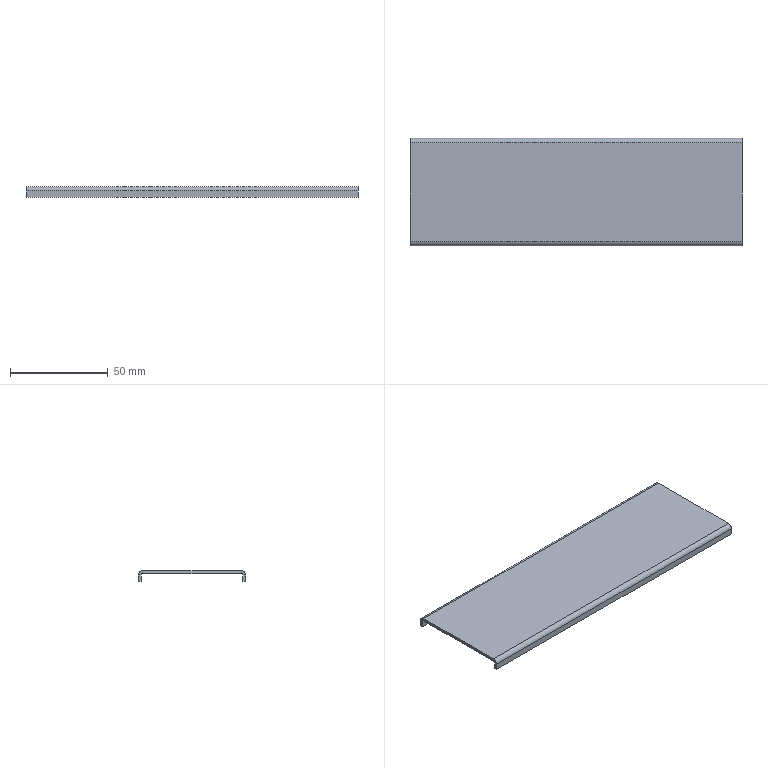Part | NX | features BREP 1 | 1 solid | 22 faces | box 170 x 55 x 5.5 mm | volume 15740 mm3 | plane 18 | cylinder 4 | commonest cylinder face diameters 1.473 x2 4.473 x2
STEP:
#1=CARTESIAN_POINT('',(85.,25.263,-1.5));
#2=VERTEX_POINT('',#1);
#3=CARTESIAN_POINT('',(-85.,25.263,-1.5));
#4=VERTEX_POINT('',#3);
#5=CARTESIAN_POINT('',(85.,25.263,-1.5));
#6=DIRECTION('',(-1.,0.,0.));
#7=VECTOR('',#6,1000.);
#8=LINE('',#5,#7);
#9=EDGE_CURVE('',#2,#4,#8,.T.);
#10=ORIENTED_EDGE('',*,*,#9,.F.);
#11=CARTESIAN_POINT('',(85.,-25.263,-1.5));
#12=VERTEX_POINT('',#11);
#13=CARTESIAN_POINT('',(85.,26.,-1.5));
#14=DIRECTION('',(0.,1.,0.));
#15=VECTOR('',#14,1000.);
#16=LINE('',#13,#15);
#17=EDGE_CURVE('',#12,#2,#16,.T.);
#18=ORIENTED_EDGE('',*,*,#17,.F.);
#19=CARTESIAN_POINT('',(-85.,-25.263,-1.5));
#20=VERTEX_POINT('',#19);
#21=CARTESIAN_POINT('',(-85.,-25.263,-1.5));
#22=DIRECTION('',(1.,0.,0.));
#23=VECTOR('',#22,1000.);
#24=LINE('',#21,#23);
#25=EDGE_CURVE('',#20,#12,#24,.T.);
#26=ORIENTED_EDGE('',*,*,#25,.F.);
#27=CARTESIAN_POINT('',(-85.,26.,-1.5));
#28=DIRECTION('',(0.,-1.,0.));
#29=VECTOR('',#28,1000.);
#30=LINE('',#27,#29);
#31=EDGE_CURVE('',#4,#20,#30,.T.);
#32=ORIENTED_EDGE('',*,*,#31,.F.);
#33=EDGE_LOOP('',(#10,#18,#26,#32));
#34=FACE_BOUND('',#33,.T.);
#35=CARTESIAN_POINT('',(0.,0.,-1.5));
#36=DIRECTION('',(0.,0.,1.));
#37=DIRECTION('',(1.,0.,0.));
#38=AXIS2_PLACEMENT_3D('',#35,#36,#37);
#39=PLANE('',#38);
#40=ADVANCED_FACE('',(#34),#39,.F.);
#41=CARTESIAN_POINT('',(85.,-25.263,0.));
#42=VERTEX_POINT('',#41);
#43=CARTESIAN_POINT('',(85.,25.263,0.));
#44=VERTEX_POINT('',#43);
#45=CARTESIAN_POINT('',(85.,26.,0.));
#46=DIRECTION('',(0.,1.,0.));
#47=VECTOR('',#46,1000.);
#48=LINE('',#45,#47);
#49=EDGE_CURVE('',#42,#44,#48,.T.);
#50=ORIENTED_EDGE('',*,*,#49,.T.);
#51=CARTESIAN_POINT('',(-85.,25.263,0.));
#52=VERTEX_POINT('',#51);
#53=CARTESIAN_POINT('',(85.,25.263,0.));
#54=DIRECTION('',(-1.,0.,0.));
#55=VECTOR('',#54,1000.);
#56=LINE('',#53,#55);
#57=EDGE_CURVE('',#44,#52,#56,.T.);
#58=ORIENTED_EDGE('',*,*,#57,.T.);
#59=CARTESIAN_POINT('',(-85.,-25.263,0.));
#60=VERTEX_POINT('',#59);
#61=CARTESIAN_POINT('',(-85.,26.,0.));
#62=DIRECTION('',(0.,-1.,0.));
#63=VECTOR('',#62,1000.);
#64=LINE('',#61,#63);
#65=EDGE_CURVE('',#52,#60,#64,.T.);
#66=ORIENTED_EDGE('',*,*,#65,.T.);
#67=CARTESIAN_POINT('',(-85.,-25.263,0.));
#68=DIRECTION('',(1.,0.,0.));
#69=VECTOR('',#68,1000.);
#70=LINE('',#67,#69);
#71=EDGE_CURVE('',#60,#42,#70,.T.);
#72=ORIENTED_EDGE('',*,*,#71,.T.);
#73=EDGE_LOOP('',(#50,#58,#66,#72));
#74=FACE_BOUND('',#73,.T.);
#75=CARTESIAN_POINT('',(0.,0.,0.));
#76=DIRECTION('',(0.,0.,1.));
#77=DIRECTION('',(1.,0.,0.));
#78=AXIS2_PLACEMENT_3D('',#75,#76,#77);
#79=PLANE('',#78);
#80=ADVANCED_FACE('',(#74),#79,.T.);
#81=ORIENTED_EDGE('',*,*,#17,.T.);
#82=CARTESIAN_POINT('',(85.,25.263,-1.5));
#83=DIRECTION('',(0.,0.,1.));
#84=VECTOR('',#83,1000.);
#85=LINE('',#82,#84);
#86=EDGE_CURVE('',#2,#44,#85,.T.);
#87=ORIENTED_EDGE('',*,*,#86,.T.);
#88=ORIENTED_EDGE('',*,*,#49,.F.);
#89=CARTESIAN_POINT('',(85.,-25.263,-1.5));
#90=DIRECTION('',(0.,0.,1.));
#91=VECTOR('',#90,1000.);
#92=LINE('',#89,#91);
#93=EDGE_CURVE('',#12,#42,#92,.T.);
#94=ORIENTED_EDGE('',*,*,#93,.F.);
#95=EDGE_LOOP('',(#81,#87,#88,#94));
#96=FACE_BOUND('',#95,.T.);
#97=CARTESIAN_POINT('',(85.,26.,-1.5));
#98=DIRECTION('',(1.,0.,0.));
#99=DIRECTION('',(0.,1.,0.));
#100=AXIS2_PLACEMENT_3D('',#97,#98,#99);
#101=PLANE('',#100);
#102=ADVANCED_FACE('',(#96),#101,.T.);
#103=CARTESIAN_POINT('',(-85.,25.263,-1.5));
#104=DIRECTION('',(0.,0.,1.));
#105=VECTOR('',#104,1000.);
#106=LINE('',#103,#105);
#107=EDGE_CURVE('',#4,#52,#106,.T.);
#108=ORIENTED_EDGE('',*,*,#107,.F.);
#109=ORIENTED_EDGE('',*,*,#31,.T.);
#110=CARTESIAN_POINT('',(-85.,-25.263,-1.5));
#111=DIRECTION('',(0.,0.,1.));
#112=VECTOR('',#111,1000.);
#113=LINE('',#110,#112);
#114=EDGE_CURVE('',#20,#60,#113,.T.);
#115=ORIENTED_EDGE('',*,*,#114,.T.);
#116=ORIENTED_EDGE('',*,*,#65,.F.);
#117=EDGE_LOOP('',(#108,#109,#115,#116));
#118=FACE_BOUND('',#117,.T.);
#119=CARTESIAN_POINT('',(-85.,26.,-1.5));
#120=DIRECTION('',(-1.,0.,0.));
#121=DIRECTION('',(0.,0.,1.));
#122=AXIS2_PLACEMENT_3D('',#119,#120,#121);
#123=PLANE('',#122);
#124=ADVANCED_FACE('',(#118),#123,.T.);
#125=CARTESIAN_POINT('',(85.,-26.,-2.237));
#126=VERTEX_POINT('',#125);
#127=CARTESIAN_POINT('',(85.,-27.5,-2.237));
#128=VERTEX_POINT('',#127);
#129=CARTESIAN_POINT('',(85.,-26.,-2.237));
#130=DIRECTION('',(0.,-1.,0.));
#131=VECTOR('',#130,1000.);
#132=LINE('',#129,#131);
#133=EDGE_CURVE('',#126,#128,#132,.T.);
#134=ORIENTED_EDGE('',*,*,#133,.F.);
#135=CARTESIAN_POINT('',(85.,-25.263,-2.237));
#136=DIRECTION('',(1.,0.,0.));
#137=DIRECTION('',(0.,0.,1.));
#138=AXIS2_PLACEMENT_3D('',#135,#136,#137);
#139=CIRCLE('',#138,0.7366);
#140=EDGE_CURVE('',#12,#126,#139,.T.);
#141=ORIENTED_EDGE('',*,*,#140,.F.);
#142=ORIENTED_EDGE('',*,*,#93,.T.);
#143=CARTESIAN_POINT('',(85.,-25.263,-2.237));
#144=DIRECTION('',(1.,0.,0.));
#145=DIRECTION('',(0.,0.,1.));
#146=AXIS2_PLACEMENT_3D('',#143,#144,#145);
#147=CIRCLE('',#146,2.237);
#148=EDGE_CURVE('',#42,#128,#147,.T.);
#149=ORIENTED_EDGE('',*,*,#148,.T.);
#150=EDGE_LOOP('',(#134,#141,#142,#149));
#151=FACE_BOUND('',#150,.T.);
#152=CARTESIAN_POINT('',(85.,-25.263,-2.237));
#153=DIRECTION('',(1.,0.,0.));
#154=DIRECTION('',(0.,1.,0.));
#155=AXIS2_PLACEMENT_3D('',#152,#153,#154);
#156=PLANE('',#155);
#157=ADVANCED_FACE('',(#151),#156,.T.);
#158=CARTESIAN_POINT('',(-85.,-26.,-2.237));
#159=VERTEX_POINT('',#158);
#160=CARTESIAN_POINT('',(-85.,-25.263,-2.237));
#161=DIRECTION('',(-1.,0.,0.));
#162=DIRECTION('',(0.,0.,1.));
#163=AXIS2_PLACEMENT_3D('',#160,#161,#162);
#164=CIRCLE('',#163,0.7366);
#165=EDGE_CURVE('',#159,#20,#164,.T.);
#166=ORIENTED_EDGE('',*,*,#165,.F.);
#167=CARTESIAN_POINT('',(-85.,-27.5,-2.237));
#168=VERTEX_POINT('',#167);
#169=CARTESIAN_POINT('',(-85.,-26.,-2.237));
#170=DIRECTION('',(0.,-1.,0.));
#171=VECTOR('',#170,1000.);
#172=LINE('',#169,#171);
#173=EDGE_CURVE('',#159,#168,#172,.T.);
#174=ORIENTED_EDGE('',*,*,#173,.T.);
#175=CARTESIAN_POINT('',(-85.,-25.263,-2.237));
#176=DIRECTION('',(-1.,0.,0.));
#177=DIRECTION('',(0.,0.,1.));
#178=AXIS2_PLACEMENT_3D('',#175,#176,#177);
#179=CIRCLE('',#178,2.237);
#180=EDGE_CURVE('',#168,#60,#179,.T.);
#181=ORIENTED_EDGE('',*,*,#180,.T.);
#182=ORIENTED_EDGE('',*,*,#114,.F.);
#183=EDGE_LOOP('',(#166,#174,#181,#182));
#184=FACE_BOUND('',#183,.T.);
#185=CARTESIAN_POINT('',(-85.,-25.263,-2.237));
#186=DIRECTION('',(1.,0.,0.));
#187=DIRECTION('',(0.,1.,0.));
#188=AXIS2_PLACEMENT_3D('',#185,#186,#187);
#189=PLANE('',#188);
#190=ADVANCED_FACE('',(#184),#189,.F.);
#191=ORIENTED_EDGE('',*,*,#71,.F.);
#192=ORIENTED_EDGE('',*,*,#180,.F.);
#193=CARTESIAN_POINT('',(0.,-27.5,-2.237));
#194=DIRECTION('',(-1.,0.,0.));
#195=VECTOR('',#194,1000.);
#196=LINE('',#193,#195);
#197=EDGE_CURVE('',#128,#168,#196,.T.);
#198=ORIENTED_EDGE('',*,*,#197,.F.);
#199=ORIENTED_EDGE('',*,*,#148,.F.);
#200=EDGE_LOOP('',(#191,#192,#198,#199));
#201=FACE_BOUND('',#200,.T.);
#202=CARTESIAN_POINT('',(-85.,-25.263,-2.237));
#203=DIRECTION('',(-1.,0.,0.));
#204=DIRECTION('',(0.,-1.,0.));
#205=AXIS2_PLACEMENT_3D('',#202,#203,#204);
#206=CYLINDRICAL_SURFACE('',#205,2.237);
#207=ADVANCED_FACE('',(#201),#206,.T.);
#208=ORIENTED_EDGE('',*,*,#25,.T.);
#209=ORIENTED_EDGE('',*,*,#140,.T.);
#210=CARTESIAN_POINT('',(85.,-26.,-2.237));
#211=DIRECTION('',(-1.,0.,0.));
#212=VECTOR('',#211,1000.);
#213=LINE('',#210,#212);
#214=EDGE_CURVE('',#126,#159,#213,.T.);
#215=ORIENTED_EDGE('',*,*,#214,.T.);
#216=ORIENTED_EDGE('',*,*,#165,.T.);
#217=EDGE_LOOP('',(#208,#209,#215,#216));
#218=FACE_BOUND('',#217,.T.);
#219=CARTESIAN_POINT('',(-85.,-25.263,-2.237));
#220=DIRECTION('',(-1.,0.,0.));
#221=DIRECTION('',(0.,-1.,0.));
#222=AXIS2_PLACEMENT_3D('',#219,#220,#221);
#223=CYLINDRICAL_SURFACE('',#222,0.7366);
#224=ADVANCED_FACE('',(#218),#223,.F.);
#225=CARTESIAN_POINT('',(-85.,-27.5,-5.5));
#226=VERTEX_POINT('',#225);
#227=CARTESIAN_POINT('',(-85.,-27.5,-1.5));
#228=DIRECTION('',(0.,0.,1.));
#229=VECTOR('',#228,1000.);
#230=LINE('',#227,#229);
#231=EDGE_CURVE('',#226,#168,#230,.T.);
#232=ORIENTED_EDGE('',*,*,#231,.T.);
#233=ORIENTED_EDGE('',*,*,#173,.F.);
#234=CARTESIAN_POINT('',(-85.,-26.,-5.5));
#235=VERTEX_POINT('',#234);
#236=CARTESIAN_POINT('',(-85.,-26.,-1.5));
#237=DIRECTION('',(0.,0.,1.));
#238=VECTOR('',#237,1000.);
#239=LINE('',#236,#238);
#240=EDGE_CURVE('',#235,#159,#239,.T.);
#241=ORIENTED_EDGE('',*,*,#240,.F.);
#242=CARTESIAN_POINT('',(-85.,-27.5,-5.5));
#243=DIRECTION('',(0.,1.,0.));
#244=VECTOR('',#243,1000.);
#245=LINE('',#242,#244);
#246=EDGE_CURVE('',#226,#235,#245,.T.);
#247=ORIENTED_EDGE('',*,*,#246,.F.);
#248=EDGE_LOOP('',(#232,#233,#241,#247));
#249=FACE_BOUND('',#248,.T.);
#250=CARTESIAN_POINT('',(-85.,-27.5,-1.5));
#251=DIRECTION('',(-1.,0.,0.));
#252=DIRECTION('',(0.,0.,1.));
#253=AXIS2_PLACEMENT_3D('',#250,#251,#252);
#254=PLANE('',#253);
#255=ADVANCED_FACE('',(#249),#254,.T.);
#256=CARTESIAN_POINT('',(85.,-26.,-5.5));
#257=VERTEX_POINT('',#256);
#258=CARTESIAN_POINT('',(85.,-26.,-5.5));
#259=DIRECTION('',(0.,0.,-1.));
#260=VECTOR('',#259,1000.);
#261=LINE('',#258,#260);
#262=EDGE_CURVE('',#126,#257,#261,.T.);
#263=ORIENTED_EDGE('',*,*,#262,.F.);
#264=ORIENTED_EDGE('',*,*,#133,.T.);
#265=CARTESIAN_POINT('',(85.,-27.5,-5.5));
#266=VERTEX_POINT('',#265);
#267=CARTESIAN_POINT('',(85.,-27.5,-5.5));
#268=DIRECTION('',(0.,0.,-1.));
#269=VECTOR('',#268,1000.);
#270=LINE('',#267,#269);
#271=EDGE_CURVE('',#128,#266,#270,.T.);
#272=ORIENTED_EDGE('',*,*,#271,.T.);
#273=CARTESIAN_POINT('',(85.,-27.5,-5.5));
#274=DIRECTION('',(0.,1.,0.));
#275=VECTOR('',#274,1000.);
#276=LINE('',#273,#275);
#277=EDGE_CURVE('',#266,#257,#276,.T.);
#278=ORIENTED_EDGE('',*,*,#277,.T.);
#279=EDGE_LOOP('',(#263,#264,#272,#278));
#280=FACE_BOUND('',#279,.T.);
#281=CARTESIAN_POINT('',(85.,-27.5,-5.5));
#282=DIRECTION('',(1.,0.,0.));
#283=DIRECTION('',(0.,0.,1.));
#284=AXIS2_PLACEMENT_3D('',#281,#282,#283);
#285=PLANE('',#284);
#286=ADVANCED_FACE('',(#280),#285,.T.);
#287=ORIENTED_EDGE('',*,*,#271,.F.);
#288=ORIENTED_EDGE('',*,*,#197,.T.);
#289=ORIENTED_EDGE('',*,*,#231,.F.);
#290=CARTESIAN_POINT('',(-85.,-27.5,-5.5));
#291=DIRECTION('',(-1.,0.,0.));
#292=VECTOR('',#291,1000.);
#293=LINE('',#290,#292);
#294=EDGE_CURVE('',#266,#226,#293,.T.);
#295=ORIENTED_EDGE('',*,*,#294,.F.);
#296=EDGE_LOOP('',(#287,#288,#289,#295));
#297=FACE_BOUND('',#296,.T.);
#298=CARTESIAN_POINT('',(0.,-27.5,0.));
#299=DIRECTION('',(0.,-1.,0.));
#300=DIRECTION('',(-1.,0.,0.));
#301=AXIS2_PLACEMENT_3D('',#298,#299,#300);
#302=PLANE('',#301);
#303=ADVANCED_FACE('',(#297),#302,.T.);
#304=ORIENTED_EDGE('',*,*,#214,.F.);
#305=ORIENTED_EDGE('',*,*,#262,.T.);
#306=CARTESIAN_POINT('',(-85.,-26.,-5.5));
#307=DIRECTION('',(-1.,0.,0.));
#308=VECTOR('',#307,1000.);
#309=LINE('',#306,#308);
#310=EDGE_CURVE('',#257,#235,#309,.T.);
#311=ORIENTED_EDGE('',*,*,#310,.T.);
#312=ORIENTED_EDGE('',*,*,#240,.T.);
#313=EDGE_LOOP('',(#304,#305,#311,#312));
#314=FACE_BOUND('',#313,.T.);
#315=CARTESIAN_POINT('',(0.,-26.,0.));
#316=DIRECTION('',(0.,-1.,0.));
#317=DIRECTION('',(-1.,0.,0.));
#318=AXIS2_PLACEMENT_3D('',#315,#316,#317);
#319=PLANE('',#318);
#320=ADVANCED_FACE('',(#314),#319,.F.);
#321=ORIENTED_EDGE('',*,*,#310,.F.);
#322=ORIENTED_EDGE('',*,*,#277,.F.);
#323=ORIENTED_EDGE('',*,*,#294,.T.);
#324=ORIENTED_EDGE('',*,*,#246,.T.);
#325=EDGE_LOOP('',(#321,#322,#323,#324));
#326=FACE_BOUND('',#325,.T.);
#327=CARTESIAN_POINT('',(-85.,-27.5,-5.5));
#328=DIRECTION('',(0.,0.,-1.));
#329=DIRECTION('',(0.,-1.,0.));
#330=AXIS2_PLACEMENT_3D('',#327,#328,#329);
#331=PLANE('',#330);
#332=ADVANCED_FACE('',(#326),#331,.T.);
#333=CARTESIAN_POINT('',(-85.,26.,-2.237));
#334=VERTEX_POINT('',#333);
#335=CARTESIAN_POINT('',(-85.,27.5,-2.237));
#336=VERTEX_POINT('',#335);
#337=CARTESIAN_POINT('',(-85.,26.,-2.237));
#338=DIRECTION('',(0.,1.,0.));
#339=VECTOR('',#338,1000.);
#340=LINE('',#337,#339);
#341=EDGE_CURVE('',#334,#336,#340,.T.);
#342=ORIENTED_EDGE('',*,*,#341,.F.);
#343=CARTESIAN_POINT('',(-85.,25.263,-2.237));
#344=DIRECTION('',(-1.,0.,0.));
#345=DIRECTION('',(0.,0.,-1.));
#346=AXIS2_PLACEMENT_3D('',#343,#344,#345);
#347=CIRCLE('',#346,0.7366);
#348=EDGE_CURVE('',#4,#334,#347,.T.);
#349=ORIENTED_EDGE('',*,*,#348,.F.);
#350=ORIENTED_EDGE('',*,*,#107,.T.);
#351=CARTESIAN_POINT('',(-85.,25.263,-2.237));
#352=DIRECTION('',(-1.,0.,0.));
#353=DIRECTION('',(0.,0.,-1.));
#354=AXIS2_PLACEMENT_3D('',#351,#352,#353);
#355=CIRCLE('',#354,2.237);
#356=EDGE_CURVE('',#52,#336,#355,.T.);
#357=ORIENTED_EDGE('',*,*,#356,.T.);
#358=EDGE_LOOP('',(#342,#349,#350,#357));
#359=FACE_BOUND('',#358,.T.);
#360=CARTESIAN_POINT('',(-85.,25.263,-2.237));
#361=DIRECTION('',(-1.,0.,0.));
#362=DIRECTION('',(0.,0.,1.));
#363=AXIS2_PLACEMENT_3D('',#360,#361,#362);
#364=PLANE('',#363);
#365=ADVANCED_FACE('',(#359),#364,.T.);
#366=CARTESIAN_POINT('',(85.,26.,-2.237));
#367=VERTEX_POINT('',#366);
#368=CARTESIAN_POINT('',(85.,25.263,-2.237));
#369=DIRECTION('',(1.,0.,0.));
#370=DIRECTION('',(0.,0.,-1.));
#371=AXIS2_PLACEMENT_3D('',#368,#369,#370);
#372=CIRCLE('',#371,0.7366);
#373=EDGE_CURVE('',#367,#2,#372,.T.);
#374=ORIENTED_EDGE('',*,*,#373,.F.);
#375=CARTESIAN_POINT('',(85.,27.5,-2.237));
#376=VERTEX_POINT('',#375);
#377=CARTESIAN_POINT('',(85.,26.,-2.237));
#378=DIRECTION('',(0.,1.,0.));
#379=VECTOR('',#378,1000.);
#380=LINE('',#377,#379);
#381=EDGE_CURVE('',#367,#376,#380,.T.);
#382=ORIENTED_EDGE('',*,*,#381,.T.);
#383=CARTESIAN_POINT('',(85.,25.263,-2.237));
#384=DIRECTION('',(1.,0.,0.));
#385=DIRECTION('',(0.,0.,-1.));
#386=AXIS2_PLACEMENT_3D('',#383,#384,#385);
#387=CIRCLE('',#386,2.237);
#388=EDGE_CURVE('',#376,#44,#387,.T.);
#389=ORIENTED_EDGE('',*,*,#388,.T.);
#390=ORIENTED_EDGE('',*,*,#86,.F.);
#391=EDGE_LOOP('',(#374,#382,#389,#390));
#392=FACE_BOUND('',#391,.T.);
#393=CARTESIAN_POINT('',(85.,25.263,-2.237));
#394=DIRECTION('',(-1.,0.,0.));
#395=DIRECTION('',(0.,0.,1.));
#396=AXIS2_PLACEMENT_3D('',#393,#394,#395);
#397=PLANE('',#396);
#398=ADVANCED_FACE('',(#392),#397,.F.);
#399=ORIENTED_EDGE('',*,*,#57,.F.);
#400=ORIENTED_EDGE('',*,*,#388,.F.);
#401=CARTESIAN_POINT('',(0.,27.5,-2.237));
#402=DIRECTION('',(-1.,0.,0.));
#403=VECTOR('',#402,1000.);
#404=LINE('',#401,#403);
#405=EDGE_CURVE('',#376,#336,#404,.T.);
#406=ORIENTED_EDGE('',*,*,#405,.T.);
#407=ORIENTED_EDGE('',*,*,#356,.F.);
#408=EDGE_LOOP('',(#399,#400,#406,#407));
#409=FACE_BOUND('',#408,.T.);
#410=CARTESIAN_POINT('',(85.,25.263,-2.237));
#411=DIRECTION('',(1.,0.,0.));
#412=DIRECTION('',(0.,1.,0.));
#413=AXIS2_PLACEMENT_3D('',#410,#411,#412);
#414=CYLINDRICAL_SURFACE('',#413,2.237);
#415=ADVANCED_FACE('',(#409),#414,.T.);
#416=ORIENTED_EDGE('',*,*,#9,.T.);
#417=ORIENTED_EDGE('',*,*,#348,.T.);
#418=CARTESIAN_POINT('',(-85.,26.,-2.237));
#419=DIRECTION('',(1.,0.,0.));
#420=VECTOR('',#419,1000.);
#421=LINE('',#418,#420);
#422=EDGE_CURVE('',#334,#367,#421,.T.);
#423=ORIENTED_EDGE('',*,*,#422,.T.);
#424=ORIENTED_EDGE('',*,*,#373,.T.);
#425=EDGE_LOOP('',(#416,#417,#423,#424));
#426=FACE_BOUND('',#425,.T.);
#427=CARTESIAN_POINT('',(85.,25.263,-2.237));
#428=DIRECTION('',(1.,0.,0.));
#429=DIRECTION('',(0.,1.,0.));
#430=AXIS2_PLACEMENT_3D('',#427,#428,#429);
#431=CYLINDRICAL_SURFACE('',#430,0.7366);
#432=ADVANCED_FACE('',(#426),#431,.F.);
#433=CARTESIAN_POINT('',(-85.,26.,-5.5));
#434=VERTEX_POINT('',#433);
#435=CARTESIAN_POINT('',(-85.,26.,-1.5));
#436=DIRECTION('',(0.,0.,-1.));
#437=VECTOR('',#436,1000.);
#438=LINE('',#435,#437);
#439=EDGE_CURVE('',#334,#434,#438,.T.);
#440=ORIENTED_EDGE('',*,*,#439,.F.);
#441=ORIENTED_EDGE('',*,*,#341,.T.);
#442=CARTESIAN_POINT('',(-85.,27.5,-5.5));
#443=VERTEX_POINT('',#442);
#444=CARTESIAN_POINT('',(-85.,27.5,-1.5));
#445=DIRECTION('',(0.,0.,-1.));
#446=VECTOR('',#445,1000.);
#447=LINE('',#444,#446);
#448=EDGE_CURVE('',#336,#443,#447,.T.);
#449=ORIENTED_EDGE('',*,*,#448,.T.);
#450=CARTESIAN_POINT('',(-85.,27.5,-5.5));
#451=DIRECTION('',(0.,-1.,0.));
#452=VECTOR('',#451,1000.);
#453=LINE('',#450,#452);
#454=EDGE_CURVE('',#443,#434,#453,.T.);
#455=ORIENTED_EDGE('',*,*,#454,.T.);
#456=EDGE_LOOP('',(#440,#441,#449,#455));
#457=FACE_BOUND('',#456,.T.);
#458=CARTESIAN_POINT('',(-85.,27.5,-1.5));
#459=DIRECTION('',(-1.,0.,0.));
#460=DIRECTION('',(0.,0.,1.));
#461=AXIS2_PLACEMENT_3D('',#458,#459,#460);
#462=PLANE('',#461);
#463=ADVANCED_FACE('',(#457),#462,.T.);
#464=CARTESIAN_POINT('',(85.,27.5,-5.5));
#465=VERTEX_POINT('',#464);
#466=CARTESIAN_POINT('',(85.,27.5,-5.5));
#467=DIRECTION('',(0.,0.,1.));
#468=VECTOR('',#467,1000.);
#469=LINE('',#466,#468);
#470=EDGE_CURVE('',#465,#376,#469,.T.);
#471=ORIENTED_EDGE('',*,*,#470,.T.);
#472=ORIENTED_EDGE('',*,*,#381,.F.);
#473=CARTESIAN_POINT('',(85.,26.,-5.5));
#474=VERTEX_POINT('',#473);
#475=CARTESIAN_POINT('',(85.,26.,-5.5));
#476=DIRECTION('',(0.,0.,1.));
#477=VECTOR('',#476,1000.);
#478=LINE('',#475,#477);
#479=EDGE_CURVE('',#474,#367,#478,.T.);
#480=ORIENTED_EDGE('',*,*,#479,.F.);
#481=CARTESIAN_POINT('',(85.,27.5,-5.5));
#482=DIRECTION('',(0.,-1.,0.));
#483=VECTOR('',#482,1000.);
#484=LINE('',#481,#483);
#485=EDGE_CURVE('',#465,#474,#484,.T.);
#486=ORIENTED_EDGE('',*,*,#485,.F.);
#487=EDGE_LOOP('',(#471,#472,#480,#486));
#488=FACE_BOUND('',#487,.T.);
#489=CARTESIAN_POINT('',(85.,27.5,-5.5));
#490=DIRECTION('',(1.,0.,0.));
#491=DIRECTION('',(0.,0.,1.));
#492=AXIS2_PLACEMENT_3D('',#489,#490,#491);
#493=PLANE('',#492);
#494=ADVANCED_FACE('',(#488),#493,.T.);
#495=ORIENTED_EDGE('',*,*,#405,.F.);
#496=ORIENTED_EDGE('',*,*,#470,.F.);
#497=CARTESIAN_POINT('',(-85.,27.5,-5.5));
#498=DIRECTION('',(1.,0.,0.));
#499=VECTOR('',#498,1000.);
#500=LINE('',#497,#499);
#501=EDGE_CURVE('',#443,#465,#500,.T.);
#502=ORIENTED_EDGE('',*,*,#501,.F.);
#503=ORIENTED_EDGE('',*,*,#448,.F.);
#504=EDGE_LOOP('',(#495,#496,#502,#503));
#505=FACE_BOUND('',#504,.T.);
#506=CARTESIAN_POINT('',(0.,27.5,0.));
#507=DIRECTION('',(0.,-1.,0.));
#508=DIRECTION('',(0.,0.,-1.));
#509=AXIS2_PLACEMENT_3D('',#506,#507,#508);
#510=PLANE('',#509);
#511=ADVANCED_FACE('',(#505),#510,.F.);
#512=ORIENTED_EDGE('',*,*,#479,.T.);
#513=ORIENTED_EDGE('',*,*,#422,.F.);
#514=ORIENTED_EDGE('',*,*,#439,.T.);
#515=CARTESIAN_POINT('',(-85.,26.,-5.5));
#516=DIRECTION('',(1.,0.,0.));
#517=VECTOR('',#516,1000.);
#518=LINE('',#515,#517);
#519=EDGE_CURVE('',#434,#474,#518,.T.);
#520=ORIENTED_EDGE('',*,*,#519,.T.);
#521=EDGE_LOOP('',(#512,#513,#514,#520));
#522=FACE_BOUND('',#521,.T.);
#523=CARTESIAN_POINT('',(0.,26.,0.));
#524=DIRECTION('',(0.,-1.,0.));
#525=DIRECTION('',(0.,0.,-1.));
#526=AXIS2_PLACEMENT_3D('',#523,#524,#525);
#527=PLANE('',#526);
#528=ADVANCED_FACE('',(#522),#527,.T.);
#529=ORIENTED_EDGE('',*,*,#519,.F.);
#530=ORIENTED_EDGE('',*,*,#454,.F.);
#531=ORIENTED_EDGE('',*,*,#501,.T.);
#532=ORIENTED_EDGE('',*,*,#485,.T.);
#533=EDGE_LOOP('',(#529,#530,#531,#532));
#534=FACE_BOUND('',#533,.T.);
#535=CARTESIAN_POINT('',(-85.,27.5,-5.5));
#536=DIRECTION('',(0.,0.,-1.));
#537=DIRECTION('',(-1.,0.,0.));
#538=AXIS2_PLACEMENT_3D('',#535,#536,#537);
#539=PLANE('',#538);
#540=ADVANCED_FACE('',(#534),#539,.T.);
#541=CLOSED_SHELL('',(#40,#80,#102,#124,#157,#190,#207,#224,#255,#286,#303,#320,#332,#365,#398,#415,#432,#463,#494,#511,#528,#540));
#542=MANIFOLD_SOLID_BREP('',#541);
#543=(LENGTH_UNIT()NAMED_UNIT(*)SI_UNIT(.MILLI.,.METRE.));
#544=UNCERTAINTY_MEASURE_WITH_UNIT(LENGTH_MEASURE(0.00001),#543,'','');
#545=(NAMED_UNIT(*)PLANE_ANGLE_UNIT()SI_UNIT($,.RADIAN.));
#546=(NAMED_UNIT(*)SI_UNIT($,.STERADIAN.)SOLID_ANGLE_UNIT());
#547=(GEOMETRIC_REPRESENTATION_CONTEXT(3)GLOBAL_UNCERTAINTY_ASSIGNED_CONTEXT((#544))GLOBAL_UNIT_ASSIGNED_CONTEXT((#543,#545,#546))REPRESENTATION_CONTEXT('',''));
#548=ADVANCED_BREP_SHAPE_REPRESENTATION('',(#542),#547);